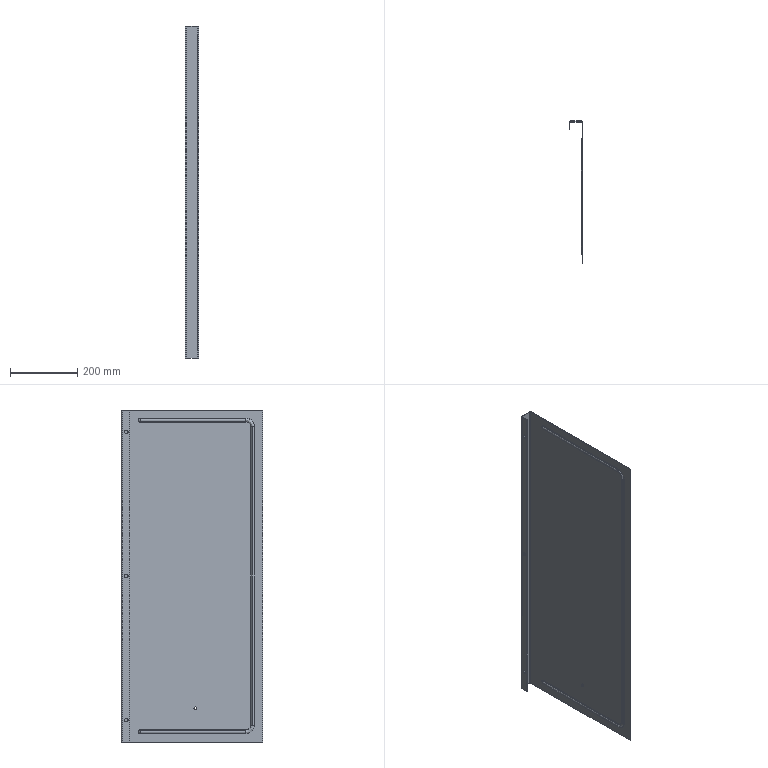Part | STEP file | 750078261 | 1 solid | 62 faces | box 40 x 420 x 985 mm | volume 948156 mm3 | cylinder 32 | spline 20 | plane 10 | commonest cylinder face diameters 4 x8 8 x8 10.5 x6 6 x4 10 x4 8.2 x2